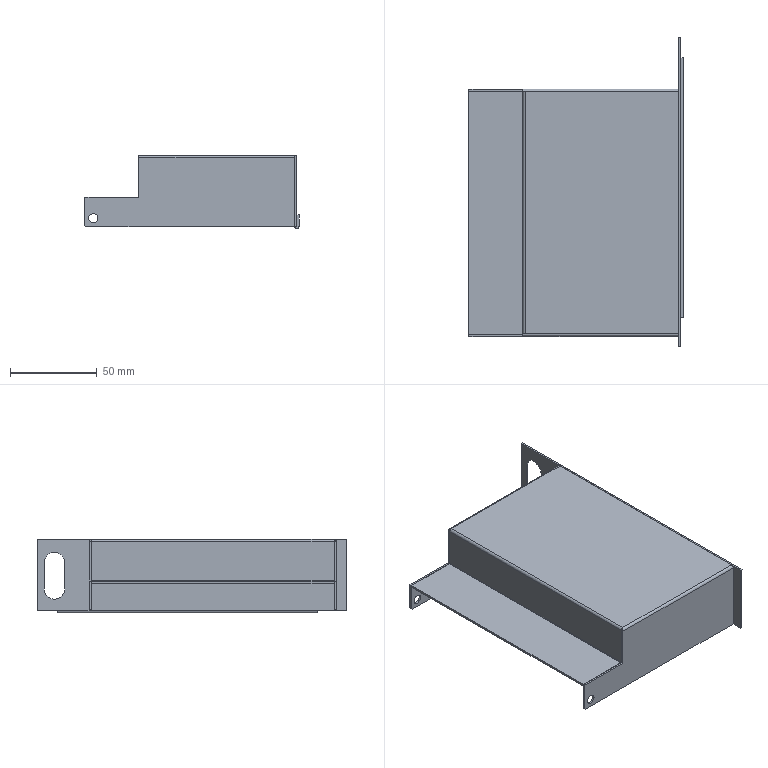Part | STEP file | 键盘盒-03^TY.NE-0002-01-014A 键盘盒-dddeger | 2 solids | 80 faces | box 123.3 x 178.4 x 42.25 mm | volume 43523 mm3 | plane 57 | cylinder 23 | commonest cylinder face diameters 2.5 x5 0.4 x4 2.8 x4 5.4 x4 12 x3 22 x2